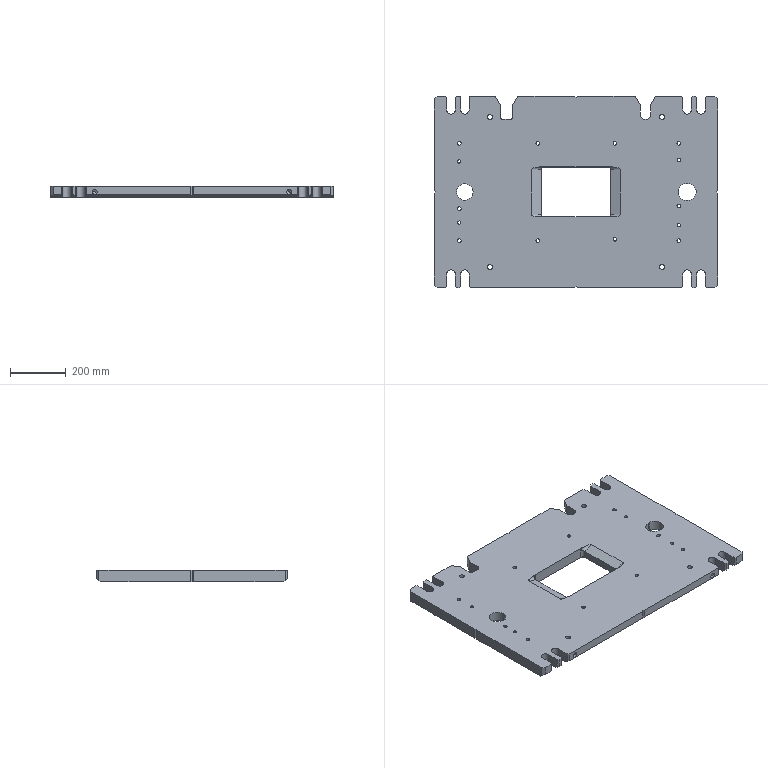Part | CATIA | 1 solid | 262 faces | box 1020 x 690 x 40 mm | volume 24770735 mm3 | plane 131 | cylinder 95 | cone 36 | commonest cylinder face diameters 20 x30 13 x20 17.5 x16 12 x8 14 x8 30 x8